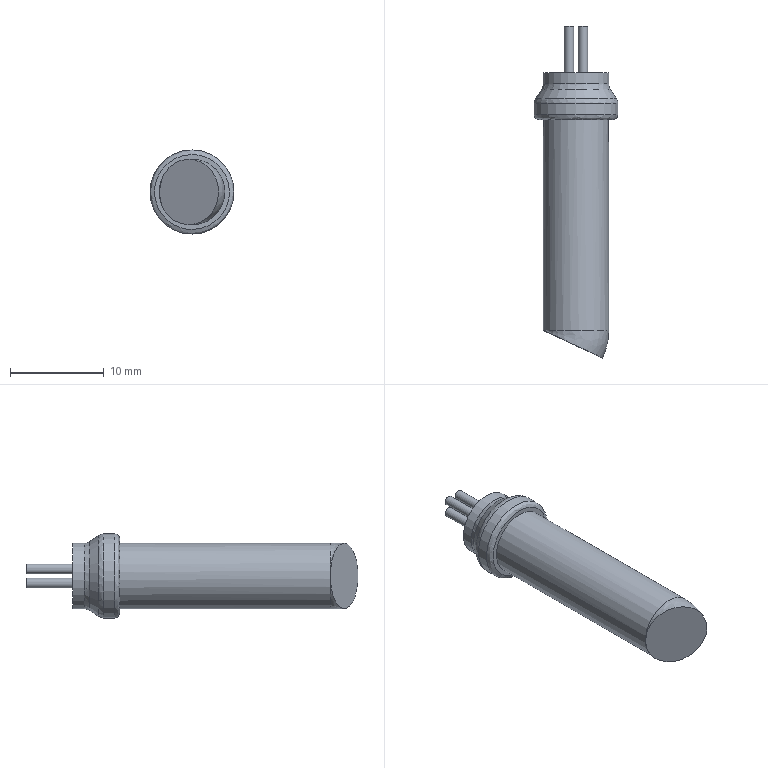Part | NX | 1 solid | 19 faces | box 9 x 35.473 x 9 mm | volume 1200 mm3 | cylinder 7 | plane 7 | spline 4 | cone 1 | commonest cylinder face diameters 1 x4 7 x2 9 x1